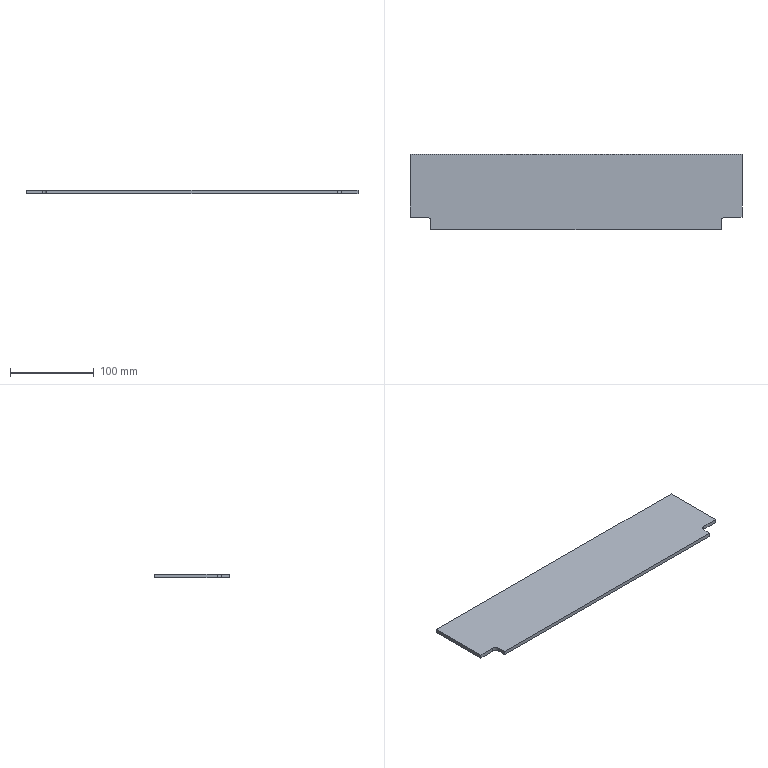Part | SolidWorks | features FlatPattern 1, SMBaseFlange 1, SheetMetal 1 | 1 solid | 12 faces | box 396 x 90 x 4.5 mm | volume 157053 mm3 | plane 10 | cylinder 2 | commonest cylinder face diameters 10 x2
STEP:
#1=CARTESIAN_POINT('',(371.,10.,0.));
#2=VERTEX_POINT('',#1);
#3=CARTESIAN_POINT('',(376.,15.,0.));
#4=VERTEX_POINT('',#3);
#5=CARTESIAN_POINT('',(376.,10.,0.));
#6=DIRECTION('',(0.,0.,-1.));
#7=DIRECTION('',(-1.,0.,0.));
#8=AXIS2_PLACEMENT_3D('',#5,#6,#7);
#9=CIRCLE('',#8,5.);
#10=EDGE_CURVE('',#2,#4,#9,.T.);
#11=ORIENTED_EDGE('',*,*,#10,.F.);
#12=CARTESIAN_POINT('',(371.,10.,-4.5));
#13=VERTEX_POINT('',#12);
#14=CARTESIAN_POINT('',(371.,10.,-4.5));
#15=DIRECTION('',(0.,0.,1.));
#16=VECTOR('',#15,1000.);
#17=LINE('',#14,#16);
#18=EDGE_CURVE('',#13,#2,#17,.T.);
#19=ORIENTED_EDGE('',*,*,#18,.F.);
#20=CARTESIAN_POINT('',(376.,15.,-4.5));
#21=VERTEX_POINT('',#20);
#22=CARTESIAN_POINT('',(376.,10.,-4.5));
#23=DIRECTION('',(0.,0.,-1.));
#24=DIRECTION('',(-1.,0.,0.));
#25=AXIS2_PLACEMENT_3D('',#22,#23,#24);
#26=CIRCLE('',#25,5.);
#27=EDGE_CURVE('',#13,#21,#26,.T.);
#28=ORIENTED_EDGE('',*,*,#27,.T.);
#29=CARTESIAN_POINT('',(376.,15.,-4.5));
#30=DIRECTION('',(0.,0.,1.));
#31=VECTOR('',#30,1000.);
#32=LINE('',#29,#31);
#33=EDGE_CURVE('',#21,#4,#32,.T.);
#34=ORIENTED_EDGE('',*,*,#33,.T.);
#35=EDGE_LOOP('',(#11,#19,#28,#34));
#36=FACE_OUTER_BOUND('',#35,.T.);
#37=CARTESIAN_POINT('',(376.,10.,-4.5));
#38=DIRECTION('',(0.,0.,1.));
#39=DIRECTION('',(1.,0.,0.));
#40=AXIS2_PLACEMENT_3D('',#37,#38,#39);
#41=CYLINDRICAL_SURFACE('',#40,5.);
#42=ADVANCED_FACE('',(#36),#41,.F.);
#43=CARTESIAN_POINT('',(371.,0.,0.));
#44=VERTEX_POINT('',#43);
#45=CARTESIAN_POINT('',(371.,10.,0.));
#46=DIRECTION('',(0.,1.,0.));
#47=VECTOR('',#46,1000.);
#48=LINE('',#45,#47);
#49=EDGE_CURVE('',#44,#2,#48,.T.);
#50=ORIENTED_EDGE('',*,*,#49,.F.);
#51=CARTESIAN_POINT('',(371.,0.,-4.5));
#52=VERTEX_POINT('',#51);
#53=CARTESIAN_POINT('',(371.,0.,-4.5));
#54=DIRECTION('',(0.,0.,1.));
#55=VECTOR('',#54,1000.);
#56=LINE('',#53,#55);
#57=EDGE_CURVE('',#52,#44,#56,.T.);
#58=ORIENTED_EDGE('',*,*,#57,.F.);
#59=CARTESIAN_POINT('',(371.,10.,-4.5));
#60=DIRECTION('',(0.,1.,0.));
#61=VECTOR('',#60,1000.);
#62=LINE('',#59,#61);
#63=EDGE_CURVE('',#52,#13,#62,.T.);
#64=ORIENTED_EDGE('',*,*,#63,.T.);
#65=ORIENTED_EDGE('',*,*,#18,.T.);
#66=EDGE_LOOP('',(#50,#58,#64,#65));
#67=FACE_OUTER_BOUND('',#66,.T.);
#68=CARTESIAN_POINT('',(371.,10.,-4.5));
#69=DIRECTION('',(1.,0.,0.));
#70=DIRECTION('',(0.,0.,-1.));
#71=AXIS2_PLACEMENT_3D('',#68,#69,#70);
#72=PLANE('',#71);
#73=ADVANCED_FACE('',(#67),#72,.T.);
#74=CARTESIAN_POINT('',(25.,0.,0.));
#75=VERTEX_POINT('',#74);
#76=CARTESIAN_POINT('',(25.,0.,0.));
#77=DIRECTION('',(1.,0.,0.));
#78=VECTOR('',#77,1000.);
#79=LINE('',#76,#78);
#80=EDGE_CURVE('',#75,#44,#79,.T.);
#81=ORIENTED_EDGE('',*,*,#80,.F.);
#82=CARTESIAN_POINT('',(25.,0.,-4.5));
#83=VERTEX_POINT('',#82);
#84=CARTESIAN_POINT('',(25.,0.,-4.5));
#85=DIRECTION('',(0.,0.,1.));
#86=VECTOR('',#85,1000.);
#87=LINE('',#84,#86);
#88=EDGE_CURVE('',#83,#75,#87,.T.);
#89=ORIENTED_EDGE('',*,*,#88,.F.);
#90=CARTESIAN_POINT('',(25.,0.,-4.5));
#91=DIRECTION('',(1.,0.,0.));
#92=VECTOR('',#91,1000.);
#93=LINE('',#90,#92);
#94=EDGE_CURVE('',#83,#52,#93,.T.);
#95=ORIENTED_EDGE('',*,*,#94,.T.);
#96=ORIENTED_EDGE('',*,*,#57,.T.);
#97=EDGE_LOOP('',(#81,#89,#95,#96));
#98=FACE_OUTER_BOUND('',#97,.T.);
#99=CARTESIAN_POINT('',(25.,0.,-4.5));
#100=DIRECTION('',(0.,-1.,0.));
#101=DIRECTION('',(0.,0.,-1.));
#102=AXIS2_PLACEMENT_3D('',#99,#100,#101);
#103=PLANE('',#102);
#104=ADVANCED_FACE('',(#98),#103,.T.);
#105=CARTESIAN_POINT('',(25.,10.,0.));
#106=VERTEX_POINT('',#105);
#107=CARTESIAN_POINT('',(25.,10.,0.));
#108=DIRECTION('',(0.,-1.,0.));
#109=VECTOR('',#108,1000.);
#110=LINE('',#107,#109);
#111=EDGE_CURVE('',#106,#75,#110,.T.);
#112=ORIENTED_EDGE('',*,*,#111,.F.);
#113=CARTESIAN_POINT('',(25.,10.,-4.5));
#114=VERTEX_POINT('',#113);
#115=CARTESIAN_POINT('',(25.,10.,-4.5));
#116=DIRECTION('',(0.,0.,1.));
#117=VECTOR('',#116,1000.);
#118=LINE('',#115,#117);
#119=EDGE_CURVE('',#114,#106,#118,.T.);
#120=ORIENTED_EDGE('',*,*,#119,.F.);
#121=CARTESIAN_POINT('',(25.,10.,-4.5));
#122=DIRECTION('',(0.,-1.,0.));
#123=VECTOR('',#122,1000.);
#124=LINE('',#121,#123);
#125=EDGE_CURVE('',#114,#83,#124,.T.);
#126=ORIENTED_EDGE('',*,*,#125,.T.);
#127=ORIENTED_EDGE('',*,*,#88,.T.);
#128=EDGE_LOOP('',(#112,#120,#126,#127));
#129=FACE_OUTER_BOUND('',#128,.T.);
#130=CARTESIAN_POINT('',(25.,10.,-4.5));
#131=DIRECTION('',(-1.,0.,0.));
#132=DIRECTION('',(0.,0.,1.));
#133=AXIS2_PLACEMENT_3D('',#130,#131,#132);
#134=PLANE('',#133);
#135=ADVANCED_FACE('',(#129),#134,.T.);
#136=CARTESIAN_POINT('',(20.,15.,0.));
#137=VERTEX_POINT('',#136);
#138=CARTESIAN_POINT('',(20.,10.,0.));
#139=DIRECTION('',(0.,0.,-1.));
#140=DIRECTION('',(1.,0.,0.));
#141=AXIS2_PLACEMENT_3D('',#138,#139,#140);
#142=CIRCLE('',#141,5.);
#143=EDGE_CURVE('',#137,#106,#142,.T.);
#144=ORIENTED_EDGE('',*,*,#143,.F.);
#145=CARTESIAN_POINT('',(20.,15.,-4.5));
#146=VERTEX_POINT('',#145);
#147=CARTESIAN_POINT('',(20.,15.,-4.5));
#148=DIRECTION('',(0.,0.,1.));
#149=VECTOR('',#148,1000.);
#150=LINE('',#147,#149);
#151=EDGE_CURVE('',#146,#137,#150,.T.);
#152=ORIENTED_EDGE('',*,*,#151,.F.);
#153=CARTESIAN_POINT('',(20.,10.,-4.5));
#154=DIRECTION('',(0.,0.,-1.));
#155=DIRECTION('',(1.,0.,0.));
#156=AXIS2_PLACEMENT_3D('',#153,#154,#155);
#157=CIRCLE('',#156,5.);
#158=EDGE_CURVE('',#146,#114,#157,.T.);
#159=ORIENTED_EDGE('',*,*,#158,.T.);
#160=ORIENTED_EDGE('',*,*,#119,.T.);
#161=EDGE_LOOP('',(#144,#152,#159,#160));
#162=FACE_OUTER_BOUND('',#161,.T.);
#163=CARTESIAN_POINT('',(20.,10.,-4.5));
#164=DIRECTION('',(0.,0.,1.));
#165=DIRECTION('',(1.,0.,0.));
#166=AXIS2_PLACEMENT_3D('',#163,#164,#165);
#167=CYLINDRICAL_SURFACE('',#166,5.);
#168=ADVANCED_FACE('',(#162),#167,.F.);
#169=CARTESIAN_POINT('',(0.,15.,0.));
#170=VERTEX_POINT('',#169);
#171=CARTESIAN_POINT('',(0.,15.,0.));
#172=DIRECTION('',(1.,0.,0.));
#173=VECTOR('',#172,1000.);
#174=LINE('',#171,#173);
#175=EDGE_CURVE('',#170,#137,#174,.T.);
#176=ORIENTED_EDGE('',*,*,#175,.F.);
#177=CARTESIAN_POINT('',(0.,15.,-4.5));
#178=VERTEX_POINT('',#177);
#179=CARTESIAN_POINT('',(0.,15.,-4.5));
#180=DIRECTION('',(0.,0.,1.));
#181=VECTOR('',#180,1000.);
#182=LINE('',#179,#181);
#183=EDGE_CURVE('',#178,#170,#182,.T.);
#184=ORIENTED_EDGE('',*,*,#183,.F.);
#185=CARTESIAN_POINT('',(0.,15.,-4.5));
#186=DIRECTION('',(1.,0.,0.));
#187=VECTOR('',#186,1000.);
#188=LINE('',#185,#187);
#189=EDGE_CURVE('',#178,#146,#188,.T.);
#190=ORIENTED_EDGE('',*,*,#189,.T.);
#191=ORIENTED_EDGE('',*,*,#151,.T.);
#192=EDGE_LOOP('',(#176,#184,#190,#191));
#193=FACE_OUTER_BOUND('',#192,.T.);
#194=CARTESIAN_POINT('',(0.,15.,-4.5));
#195=DIRECTION('',(0.,-1.,0.));
#196=DIRECTION('',(0.,0.,-1.));
#197=AXIS2_PLACEMENT_3D('',#194,#195,#196);
#198=PLANE('',#197);
#199=ADVANCED_FACE('',(#193),#198,.T.);
#200=CARTESIAN_POINT('',(0.,90.,0.));
#201=VERTEX_POINT('',#200);
#202=CARTESIAN_POINT('',(0.,15.,0.));
#203=DIRECTION('',(0.,-1.,0.));
#204=VECTOR('',#203,1000.);
#205=LINE('',#202,#204);
#206=EDGE_CURVE('',#201,#170,#205,.T.);
#207=ORIENTED_EDGE('',*,*,#206,.F.);
#208=CARTESIAN_POINT('',(0.,90.,-4.5));
#209=VERTEX_POINT('',#208);
#210=CARTESIAN_POINT('',(0.,90.,-4.5));
#211=DIRECTION('',(0.,0.,1.));
#212=VECTOR('',#211,1000.);
#213=LINE('',#210,#212);
#214=EDGE_CURVE('',#209,#201,#213,.T.);
#215=ORIENTED_EDGE('',*,*,#214,.F.);
#216=CARTESIAN_POINT('',(0.,15.,-4.5));
#217=DIRECTION('',(0.,-1.,0.));
#218=VECTOR('',#217,1000.);
#219=LINE('',#216,#218);
#220=EDGE_CURVE('',#209,#178,#219,.T.);
#221=ORIENTED_EDGE('',*,*,#220,.T.);
#222=ORIENTED_EDGE('',*,*,#183,.T.);
#223=EDGE_LOOP('',(#207,#215,#221,#222));
#224=FACE_OUTER_BOUND('',#223,.T.);
#225=CARTESIAN_POINT('',(0.,15.,-4.5));
#226=DIRECTION('',(-1.,0.,0.));
#227=DIRECTION('',(0.,-1.,0.));
#228=AXIS2_PLACEMENT_3D('',#225,#226,#227);
#229=PLANE('',#228);
#230=ADVANCED_FACE('',(#224),#229,.T.);
#231=CARTESIAN_POINT('',(396.,90.,0.));
#232=VERTEX_POINT('',#231);
#233=CARTESIAN_POINT('',(0.,90.,0.));
#234=DIRECTION('',(-1.,0.,0.));
#235=VECTOR('',#234,1000.);
#236=LINE('',#233,#235);
#237=EDGE_CURVE('',#232,#201,#236,.T.);
#238=ORIENTED_EDGE('',*,*,#237,.F.);
#239=CARTESIAN_POINT('',(396.,90.,-4.5));
#240=VERTEX_POINT('',#239);
#241=CARTESIAN_POINT('',(396.,90.,-4.5));
#242=DIRECTION('',(0.,0.,1.));
#243=VECTOR('',#242,1000.);
#244=LINE('',#241,#243);
#245=EDGE_CURVE('',#240,#232,#244,.T.);
#246=ORIENTED_EDGE('',*,*,#245,.F.);
#247=CARTESIAN_POINT('',(0.,90.,-4.5));
#248=DIRECTION('',(-1.,0.,0.));
#249=VECTOR('',#248,1000.);
#250=LINE('',#247,#249);
#251=EDGE_CURVE('',#240,#209,#250,.T.);
#252=ORIENTED_EDGE('',*,*,#251,.T.);
#253=ORIENTED_EDGE('',*,*,#214,.T.);
#254=EDGE_LOOP('',(#238,#246,#252,#253));
#255=FACE_OUTER_BOUND('',#254,.T.);
#256=CARTESIAN_POINT('',(0.,90.,-4.5));
#257=DIRECTION('',(0.,1.,0.));
#258=DIRECTION('',(0.,0.,1.));
#259=AXIS2_PLACEMENT_3D('',#256,#257,#258);
#260=PLANE('',#259);
#261=ADVANCED_FACE('',(#255),#260,.T.);
#262=CARTESIAN_POINT('',(396.,15.,0.));
#263=VERTEX_POINT('',#262);
#264=CARTESIAN_POINT('',(396.,15.,0.));
#265=DIRECTION('',(0.,1.,0.));
#266=VECTOR('',#265,1000.);
#267=LINE('',#264,#266);
#268=EDGE_CURVE('',#263,#232,#267,.T.);
#269=ORIENTED_EDGE('',*,*,#268,.F.);
#270=CARTESIAN_POINT('',(396.,15.,-4.5));
#271=VERTEX_POINT('',#270);
#272=CARTESIAN_POINT('',(396.,15.,-4.5));
#273=DIRECTION('',(0.,0.,1.));
#274=VECTOR('',#273,1000.);
#275=LINE('',#272,#274);
#276=EDGE_CURVE('',#271,#263,#275,.T.);
#277=ORIENTED_EDGE('',*,*,#276,.F.);
#278=CARTESIAN_POINT('',(396.,15.,-4.5));
#279=DIRECTION('',(0.,1.,0.));
#280=VECTOR('',#279,1000.);
#281=LINE('',#278,#280);
#282=EDGE_CURVE('',#271,#240,#281,.T.);
#283=ORIENTED_EDGE('',*,*,#282,.T.);
#284=ORIENTED_EDGE('',*,*,#245,.T.);
#285=EDGE_LOOP('',(#269,#277,#283,#284));
#286=FACE_OUTER_BOUND('',#285,.T.);
#287=CARTESIAN_POINT('',(396.,15.,-4.5));
#288=DIRECTION('',(1.,0.,0.));
#289=DIRECTION('',(0.,0.,-1.));
#290=AXIS2_PLACEMENT_3D('',#287,#288,#289);
#291=PLANE('',#290);
#292=ADVANCED_FACE('',(#286),#291,.T.);
#293=CARTESIAN_POINT('',(396.,15.,0.));
#294=DIRECTION('',(1.,0.,0.));
#295=VECTOR('',#294,1000.);
#296=LINE('',#293,#295);
#297=EDGE_CURVE('',#4,#263,#296,.T.);
#298=ORIENTED_EDGE('',*,*,#297,.F.);
#299=ORIENTED_EDGE('',*,*,#33,.F.);
#300=CARTESIAN_POINT('',(396.,15.,-4.5));
#301=DIRECTION('',(1.,0.,0.));
#302=VECTOR('',#301,1000.);
#303=LINE('',#300,#302);
#304=EDGE_CURVE('',#21,#271,#303,.T.);
#305=ORIENTED_EDGE('',*,*,#304,.T.);
#306=ORIENTED_EDGE('',*,*,#276,.T.);
#307=EDGE_LOOP('',(#298,#299,#305,#306));
#308=FACE_OUTER_BOUND('',#307,.T.);
#309=CARTESIAN_POINT('',(396.,15.,-4.5));
#310=DIRECTION('',(0.,-1.,0.));
#311=DIRECTION('',(1.,0.,0.));
#312=AXIS2_PLACEMENT_3D('',#309,#310,#311);
#313=PLANE('',#312);
#314=ADVANCED_FACE('',(#308),#313,.T.);
#315=ORIENTED_EDGE('',*,*,#27,.F.);
#316=ORIENTED_EDGE('',*,*,#63,.F.);
#317=ORIENTED_EDGE('',*,*,#94,.F.);
#318=ORIENTED_EDGE('',*,*,#125,.F.);
#319=ORIENTED_EDGE('',*,*,#158,.F.);
#320=ORIENTED_EDGE('',*,*,#189,.F.);
#321=ORIENTED_EDGE('',*,*,#220,.F.);
#322=ORIENTED_EDGE('',*,*,#251,.F.);
#323=ORIENTED_EDGE('',*,*,#282,.F.);
#324=ORIENTED_EDGE('',*,*,#304,.F.);
#325=EDGE_LOOP('',(#315,#316,#317,#318,#319,#320,#321,#322,#323,#324));
#326=FACE_OUTER_BOUND('',#325,.T.);
#327=CARTESIAN_POINT('',(376.,10.,-4.5));
#328=DIRECTION('',(0.,0.,-1.));
#329=DIRECTION('',(-1.,0.,0.));
#330=AXIS2_PLACEMENT_3D('',#327,#328,#329);
#331=PLANE('',#330);
#332=ADVANCED_FACE('',(#326),#331,.T.);
#333=ORIENTED_EDGE('',*,*,#10,.T.);
#334=ORIENTED_EDGE('',*,*,#297,.T.);
#335=ORIENTED_EDGE('',*,*,#268,.T.);
#336=ORIENTED_EDGE('',*,*,#237,.T.);
#337=ORIENTED_EDGE('',*,*,#206,.T.);
#338=ORIENTED_EDGE('',*,*,#175,.T.);
#339=ORIENTED_EDGE('',*,*,#143,.T.);
#340=ORIENTED_EDGE('',*,*,#111,.T.);
#341=ORIENTED_EDGE('',*,*,#80,.T.);
#342=ORIENTED_EDGE('',*,*,#49,.T.);
#343=EDGE_LOOP('',(#333,#334,#335,#336,#337,#338,#339,#340,#341,#342));
#344=FACE_OUTER_BOUND('',#343,.T.);
#345=CARTESIAN_POINT('',(376.,10.,0.));
#346=DIRECTION('',(0.,0.,-1.));
#347=DIRECTION('',(-1.,0.,0.));
#348=AXIS2_PLACEMENT_3D('',#345,#346,#347);
#349=PLANE('',#348);
#350=ADVANCED_FACE('',(#344),#349,.F.);
#351=CLOSED_SHELL('',(#42,#73,#104,#135,#168,#199,#230,#261,#292,#314,#332,#350));
#352=MANIFOLD_SOLID_BREP('',#351);
#353=CARTESIAN_POINT('',(0.,0.,0.));
#354=DIRECTION('',(0.,0.,1.));
#355=DIRECTION('',(1.,0.,0.));
#356=AXIS2_PLACEMENT_3D('',#353,#354,#355);
#357=(LENGTH_UNIT()NAMED_UNIT(*)SI_UNIT(.MILLI.,.METRE.));
#358=UNCERTAINTY_MEASURE_WITH_UNIT(LENGTH_MEASURE(0.00001),#357,'','');
#359=(NAMED_UNIT(*)PLANE_ANGLE_UNIT()SI_UNIT($,.RADIAN.));
#360=(NAMED_UNIT(*)SI_UNIT($,.STERADIAN.)SOLID_ANGLE_UNIT());
#361=(GEOMETRIC_REPRESENTATION_CONTEXT(3)GLOBAL_UNCERTAINTY_ASSIGNED_CONTEXT((#358))GLOBAL_UNIT_ASSIGNED_CONTEXT((#357,#359,#360))REPRESENTATION_CONTEXT('',''));
#362=ADVANCED_BREP_SHAPE_REPRESENTATION('',(#352,#356),#361);